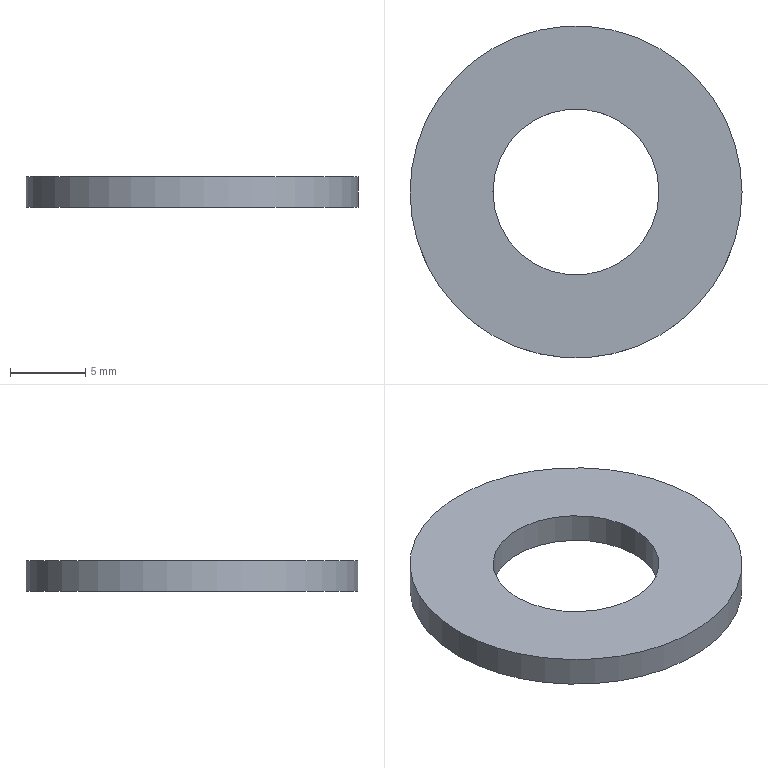Part | NX | features DATUM_CSYS 2, EXTRUDE 1, SKETCH 1 | 1 solid | 4 faces | box 22 x 22 x 2 mm | volume 570.199 mm3 | cylinder 2 | plane 2 | commonest cylinder face diameters 11 x1 22 x1
STEP:
#1=CARTESIAN_POINT('',(11.,0.,2.));
#2=VERTEX_POINT('',#1);
#3=CARTESIAN_POINT('',(0.,0.,2.));
#4=DIRECTION('',(0.,0.,1.));
#5=DIRECTION('',(1.,0.,0.));
#6=AXIS2_PLACEMENT_3D('',#3,#4,#5);
#7=CIRCLE('',#6,11.);
#8=EDGE_CURVE('',#2,#2,#7,.T.);
#9=ORIENTED_EDGE('',*,*,#8,.F.);
#10=EDGE_LOOP('',(#9));
#11=FACE_BOUND('',#10,.T.);
#12=CARTESIAN_POINT('',(11.,0.,0.));
#13=VERTEX_POINT('',#12);
#14=CARTESIAN_POINT('',(0.,0.,0.));
#15=DIRECTION('',(0.,0.,1.));
#16=DIRECTION('',(1.,0.,0.));
#17=AXIS2_PLACEMENT_3D('',#14,#15,#16);
#18=CIRCLE('',#17,11.);
#19=EDGE_CURVE('',#13,#13,#18,.T.);
#20=ORIENTED_EDGE('',*,*,#19,.T.);
#21=EDGE_LOOP('',(#20));
#22=FACE_BOUND('',#21,.T.);
#23=CARTESIAN_POINT('',(0.,0.,2.));
#24=DIRECTION('',(0.,0.,-1.));
#25=DIRECTION('',(-1.,0.,0.));
#26=AXIS2_PLACEMENT_3D('',#23,#24,#25);
#27=CYLINDRICAL_SURFACE('',#26,11.);
#28=ADVANCED_FACE('',(#11,#22),#27,.T.);
#29=CARTESIAN_POINT('',(5.5,0.,2.));
#30=VERTEX_POINT('',#29);
#31=CARTESIAN_POINT('',(0.,0.,2.));
#32=DIRECTION('',(0.,0.,1.));
#33=DIRECTION('',(1.,0.,0.));
#34=AXIS2_PLACEMENT_3D('',#31,#32,#33);
#35=CIRCLE('',#34,5.5);
#36=EDGE_CURVE('',#30,#30,#35,.T.);
#37=ORIENTED_EDGE('',*,*,#36,.T.);
#38=EDGE_LOOP('',(#37));
#39=FACE_BOUND('',#38,.T.);
#40=CARTESIAN_POINT('',(5.5,0.,0.));
#41=VERTEX_POINT('',#40);
#42=CARTESIAN_POINT('',(0.,0.,0.));
#43=DIRECTION('',(0.,0.,1.));
#44=DIRECTION('',(1.,0.,0.));
#45=AXIS2_PLACEMENT_3D('',#42,#43,#44);
#46=CIRCLE('',#45,5.5);
#47=EDGE_CURVE('',#41,#41,#46,.T.);
#48=ORIENTED_EDGE('',*,*,#47,.F.);
#49=EDGE_LOOP('',(#48));
#50=FACE_BOUND('',#49,.T.);
#51=CARTESIAN_POINT('',(0.,0.,2.));
#52=DIRECTION('',(0.,0.,-1.));
#53=DIRECTION('',(-1.,0.,0.));
#54=AXIS2_PLACEMENT_3D('',#51,#52,#53);
#55=CYLINDRICAL_SURFACE('',#54,5.5);
#56=ADVANCED_FACE('',(#39,#50),#55,.F.);
#57=ORIENTED_EDGE('',*,*,#8,.T.);
#58=EDGE_LOOP('',(#57));
#59=FACE_BOUND('',#58,.T.);
#60=ORIENTED_EDGE('',*,*,#36,.F.);
#61=EDGE_LOOP('',(#60));
#62=FACE_BOUND('',#61,.T.);
#63=CARTESIAN_POINT('',(0.,0.,2.));
#64=DIRECTION('',(0.,0.,1.));
#65=DIRECTION('',(1.,0.,0.));
#66=AXIS2_PLACEMENT_3D('',#63,#64,#65);
#67=PLANE('',#66);
#68=ADVANCED_FACE('',(#59,#62),#67,.T.);
#69=ORIENTED_EDGE('',*,*,#19,.F.);
#70=EDGE_LOOP('',(#69));
#71=FACE_BOUND('',#70,.T.);
#72=ORIENTED_EDGE('',*,*,#47,.T.);
#73=EDGE_LOOP('',(#72));
#74=FACE_BOUND('',#73,.T.);
#75=CARTESIAN_POINT('',(0.,0.,0.));
#76=DIRECTION('',(0.,0.,1.));
#77=DIRECTION('',(1.,0.,0.));
#78=AXIS2_PLACEMENT_3D('',#75,#76,#77);
#79=PLANE('',#78);
#80=ADVANCED_FACE('',(#71,#74),#79,.F.);
#81=CLOSED_SHELL('',(#28,#56,#68,#80));
#82=MANIFOLD_SOLID_BREP('',#81);
#83=(LENGTH_UNIT()NAMED_UNIT(*)SI_UNIT(.MILLI.,.METRE.));
#84=UNCERTAINTY_MEASURE_WITH_UNIT(LENGTH_MEASURE(0.00001),#83,'','');
#85=(NAMED_UNIT(*)PLANE_ANGLE_UNIT()SI_UNIT($,.RADIAN.));
#86=(NAMED_UNIT(*)SI_UNIT($,.STERADIAN.)SOLID_ANGLE_UNIT());
#87=(GEOMETRIC_REPRESENTATION_CONTEXT(3)GLOBAL_UNCERTAINTY_ASSIGNED_CONTEXT((#84))GLOBAL_UNIT_ASSIGNED_CONTEXT((#83,#85,#86))REPRESENTATION_CONTEXT('',''));
#88=ADVANCED_BREP_SHAPE_REPRESENTATION('',(#82),#87);